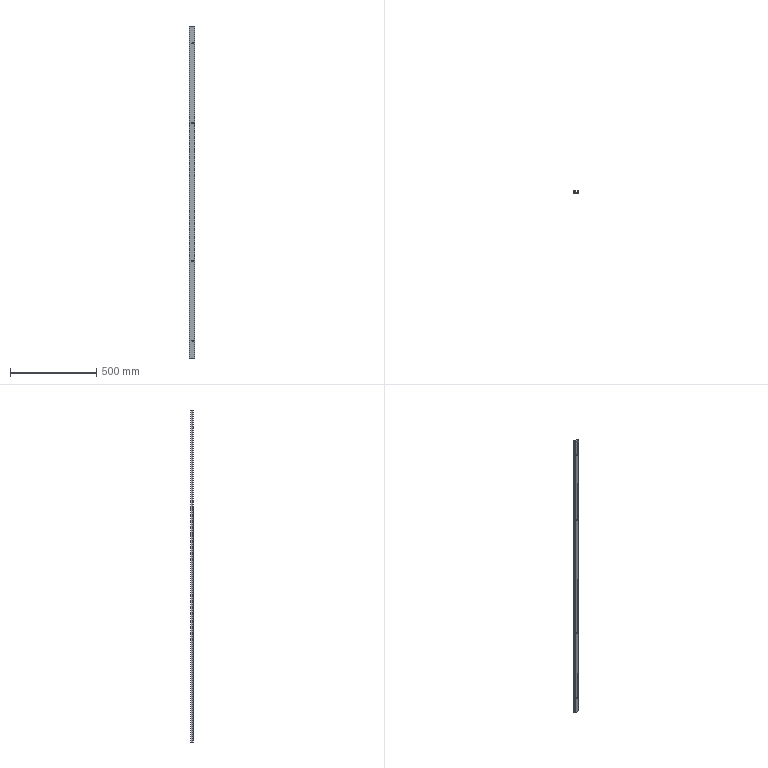Part | SolidWorks | features ICE 2, BaseBody 1, HoleWzd 1, MoveFace 1 | 1 solid | 35 faces | box 33.5 x 13.5 x 1920 mm | volume 359220 mm3 | plane 17 | cylinder 10 | cone 8 | commonest cylinder face diameters 13.44 x4 2 x3 4 x2 1.5 x1
STEP:
#1=CARTESIAN_POINT('',(20.,0.,1723.72));
#2=VERTEX_POINT('',#1);
#3=CARTESIAN_POINT('',(20.,0.,1716.28));
#4=VERTEX_POINT('',#3);
#5=CARTESIAN_POINT('',(20.,0.,1720.));
#6=DIRECTION('',(0.,-1.,0.));
#7=DIRECTION('',(0.,0.,-1.));
#8=AXIS2_PLACEMENT_3D('',#5,#6,#7);
#9=CIRCLE('',#8,3.72);
#10=EDGE_CURVE('',#2,#4,#9,.T.);
#11=ORIENTED_EDGE('',*,*,#10,.T.);
#12=CARTESIAN_POINT('',(20.,3.,1713.28));
#13=VERTEX_POINT('',#12);
#14=CARTESIAN_POINT('',(20.,3.,1713.28));
#15=DIRECTION('',(0.,0.7071,-0.7071));
#16=VECTOR('',#15,1000.);
#17=LINE('',#14,#16);
#18=EDGE_CURVE('',#4,#13,#17,.T.);
#19=ORIENTED_EDGE('',*,*,#18,.T.);
#20=CARTESIAN_POINT('',(20.,3.,1726.72));
#21=VERTEX_POINT('',#20);
#22=CARTESIAN_POINT('',(20.,3.,1720.));
#23=DIRECTION('',(0.,1.,0.));
#24=DIRECTION('',(0.,0.,1.));
#25=AXIS2_PLACEMENT_3D('',#22,#23,#24);
#26=CIRCLE('',#25,6.72);
#27=EDGE_CURVE('',#13,#21,#26,.T.);
#28=ORIENTED_EDGE('',*,*,#27,.T.);
#29=CARTESIAN_POINT('',(20.,3.,1726.72));
#30=DIRECTION('',(0.,0.7071,0.7071));
#31=VECTOR('',#30,1000.);
#32=LINE('',#29,#31);
#33=EDGE_CURVE('',#2,#21,#32,.T.);
#34=ORIENTED_EDGE('',*,*,#33,.F.);
#35=EDGE_LOOP('',(#11,#19,#28,#34));
#36=FACE_OUTER_BOUND('',#35,.T.);
#37=CARTESIAN_POINT('',(20.,3.,1720.));
#38=DIRECTION('',(0.,1.,0.));
#39=DIRECTION('',(0.,0.,1.));
#40=AXIS2_PLACEMENT_3D('',#37,#38,#39);
#41=CONICAL_SURFACE('',#40,6.72,0.7854);
#42=ADVANCED_FACE('',(#36),#41,.F.);
#43=CARTESIAN_POINT('',(20.,0.,3.72));
#44=VERTEX_POINT('',#43);
#45=CARTESIAN_POINT('',(20.,0.,-3.72));
#46=VERTEX_POINT('',#45);
#47=CARTESIAN_POINT('',(20.,0.,0.));
#48=DIRECTION('',(0.,-1.,0.));
#49=DIRECTION('',(0.,0.,-1.));
#50=AXIS2_PLACEMENT_3D('',#47,#48,#49);
#51=CIRCLE('',#50,3.72);
#52=EDGE_CURVE('',#44,#46,#51,.T.);
#53=ORIENTED_EDGE('',*,*,#52,.T.);
#54=CARTESIAN_POINT('',(20.,3.,-6.72));
#55=VERTEX_POINT('',#54);
#56=CARTESIAN_POINT('',(20.,3.,-6.72));
#57=DIRECTION('',(0.,0.7071,-0.7071));
#58=VECTOR('',#57,1000.);
#59=LINE('',#56,#58);
#60=EDGE_CURVE('',#46,#55,#59,.T.);
#61=ORIENTED_EDGE('',*,*,#60,.T.);
#62=CARTESIAN_POINT('',(20.,3.,6.72));
#63=VERTEX_POINT('',#62);
#64=CARTESIAN_POINT('',(20.,3.,0.));
#65=DIRECTION('',(0.,1.,0.));
#66=DIRECTION('',(0.,0.,1.));
#67=AXIS2_PLACEMENT_3D('',#64,#65,#66);
#68=CIRCLE('',#67,6.72);
#69=EDGE_CURVE('',#55,#63,#68,.T.);
#70=ORIENTED_EDGE('',*,*,#69,.T.);
#71=CARTESIAN_POINT('',(20.,3.,6.72));
#72=DIRECTION('',(0.,0.7071,0.7071));
#73=VECTOR('',#72,1000.);
#74=LINE('',#71,#73);
#75=EDGE_CURVE('',#44,#63,#74,.T.);
#76=ORIENTED_EDGE('',*,*,#75,.F.);
#77=EDGE_LOOP('',(#53,#61,#70,#76));
#78=FACE_OUTER_BOUND('',#77,.T.);
#79=CARTESIAN_POINT('',(20.,3.,0.));
#80=DIRECTION('',(0.,1.,0.));
#81=DIRECTION('',(0.,0.,1.));
#82=AXIS2_PLACEMENT_3D('',#79,#80,#81);
#83=CONICAL_SURFACE('',#82,6.72,0.7854);
#84=ADVANCED_FACE('',(#78),#83,.F.);
#85=CARTESIAN_POINT('',(20.,0.,463.72));
#86=VERTEX_POINT('',#85);
#87=CARTESIAN_POINT('',(20.,0.,456.28));
#88=VERTEX_POINT('',#87);
#89=CARTESIAN_POINT('',(20.,0.,460.));
#90=DIRECTION('',(0.,-1.,0.));
#91=DIRECTION('',(0.,0.,-1.));
#92=AXIS2_PLACEMENT_3D('',#89,#90,#91);
#93=CIRCLE('',#92,3.72);
#94=EDGE_CURVE('',#86,#88,#93,.T.);
#95=ORIENTED_EDGE('',*,*,#94,.T.);
#96=CARTESIAN_POINT('',(20.,3.,453.28));
#97=VERTEX_POINT('',#96);
#98=CARTESIAN_POINT('',(20.,3.,453.28));
#99=DIRECTION('',(0.,0.7071,-0.7071));
#100=VECTOR('',#99,1000.);
#101=LINE('',#98,#100);
#102=EDGE_CURVE('',#88,#97,#101,.T.);
#103=ORIENTED_EDGE('',*,*,#102,.T.);
#104=CARTESIAN_POINT('',(20.,3.,466.72));
#105=VERTEX_POINT('',#104);
#106=CARTESIAN_POINT('',(20.,3.,460.));
#107=DIRECTION('',(0.,1.,0.));
#108=DIRECTION('',(0.,0.,1.));
#109=AXIS2_PLACEMENT_3D('',#106,#107,#108);
#110=CIRCLE('',#109,6.72);
#111=EDGE_CURVE('',#97,#105,#110,.T.);
#112=ORIENTED_EDGE('',*,*,#111,.T.);
#113=CARTESIAN_POINT('',(20.,3.,466.72));
#114=DIRECTION('',(0.,0.7071,0.7071));
#115=VECTOR('',#114,1000.);
#116=LINE('',#113,#115);
#117=EDGE_CURVE('',#86,#105,#116,.T.);
#118=ORIENTED_EDGE('',*,*,#117,.F.);
#119=EDGE_LOOP('',(#95,#103,#112,#118));
#120=FACE_OUTER_BOUND('',#119,.T.);
#121=CARTESIAN_POINT('',(20.,3.,460.));
#122=DIRECTION('',(0.,1.,0.));
#123=DIRECTION('',(0.,0.,1.));
#124=AXIS2_PLACEMENT_3D('',#121,#122,#123);
#125=CONICAL_SURFACE('',#124,6.72,0.7854);
#126=ADVANCED_FACE('',(#120),#125,.F.);
#127=CARTESIAN_POINT('',(20.,0.,1263.72));
#128=VERTEX_POINT('',#127);
#129=CARTESIAN_POINT('',(20.,0.,1256.28));
#130=VERTEX_POINT('',#129);
#131=CARTESIAN_POINT('',(20.,0.,1260.));
#132=DIRECTION('',(0.,-1.,0.));
#133=DIRECTION('',(0.,0.,-1.));
#134=AXIS2_PLACEMENT_3D('',#131,#132,#133);
#135=CIRCLE('',#134,3.72);
#136=EDGE_CURVE('',#128,#130,#135,.T.);
#137=ORIENTED_EDGE('',*,*,#136,.T.);
#138=CARTESIAN_POINT('',(20.,3.,1253.28));
#139=VERTEX_POINT('',#138);
#140=CARTESIAN_POINT('',(20.,3.,1253.28));
#141=DIRECTION('',(0.,0.7071,-0.7071));
#142=VECTOR('',#141,1000.);
#143=LINE('',#140,#142);
#144=EDGE_CURVE('',#130,#139,#143,.T.);
#145=ORIENTED_EDGE('',*,*,#144,.T.);
#146=CARTESIAN_POINT('',(20.,3.,1266.72));
#147=VERTEX_POINT('',#146);
#148=CARTESIAN_POINT('',(20.,3.,1260.));
#149=DIRECTION('',(0.,1.,0.));
#150=DIRECTION('',(0.,0.,1.));
#151=AXIS2_PLACEMENT_3D('',#148,#149,#150);
#152=CIRCLE('',#151,6.72);
#153=EDGE_CURVE('',#139,#147,#152,.T.);
#154=ORIENTED_EDGE('',*,*,#153,.T.);
#155=CARTESIAN_POINT('',(20.,3.,1266.72));
#156=DIRECTION('',(0.,0.7071,0.7071));
#157=VECTOR('',#156,1000.);
#158=LINE('',#155,#157);
#159=EDGE_CURVE('',#128,#147,#158,.T.);
#160=ORIENTED_EDGE('',*,*,#159,.F.);
#161=EDGE_LOOP('',(#137,#145,#154,#160));
#162=FACE_OUTER_BOUND('',#161,.T.);
#163=CARTESIAN_POINT('',(20.,3.,1260.));
#164=DIRECTION('',(0.,1.,0.));
#165=DIRECTION('',(0.,0.,1.));
#166=AXIS2_PLACEMENT_3D('',#163,#164,#165);
#167=CONICAL_SURFACE('',#166,6.72,0.7854);
#168=ADVANCED_FACE('',(#162),#167,.F.);
#169=CARTESIAN_POINT('',(24.5,10.5,1255.009));
#170=VERTEX_POINT('',#169);
#171=CARTESIAN_POINT('',(24.5,10.5,464.991));
#172=VERTEX_POINT('',#171);
#173=CARTESIAN_POINT('',(24.5,10.5,-100.));
#174=DIRECTION('',(0.,0.,-1.));
#175=VECTOR('',#174,1000.);
#176=LINE('',#173,#175);
#177=EDGE_CURVE('',#170,#172,#176,.T.);
#178=ORIENTED_EDGE('',*,*,#177,.F.);
#179=CARTESIAN_POINT('',(24.5,10.5,1264.991));
#180=VERTEX_POINT('',#179);
#181=CARTESIAN_POINT('',(24.5,10.5,1255.009));
#182=CARTESIAN_POINT('',(24.5,10.64,1255.009));
#183=CARTESIAN_POINT('',(24.514,10.776,1255.022));
#184=CARTESIAN_POINT('',(24.57,11.042,1255.073));
#185=CARTESIAN_POINT('',(24.611,11.171,1255.111));
#186=CARTESIAN_POINT('',(24.713,11.408,1255.209));
#187=CARTESIAN_POINT('',(24.775,11.519,1255.27));
#188=CARTESIAN_POINT('',(24.908,11.717,1255.409));
#189=CARTESIAN_POINT('',(24.981,11.806,1255.488));
#190=CARTESIAN_POINT('',(25.207,12.042,1255.746));
#191=CARTESIAN_POINT('',(25.363,12.155,1255.942));
#192=CARTESIAN_POINT('',(25.665,12.326,1256.376));
#193=CARTESIAN_POINT('',(25.806,12.38,1256.605));
#194=CARTESIAN_POINT('',(26.061,12.456,1257.084));
#195=CARTESIAN_POINT('',(26.176,12.476,1257.337));
#196=CARTESIAN_POINT('',(26.372,12.498,1257.849));
#197=CARTESIAN_POINT('',(26.454,12.501,1258.109));
#198=CARTESIAN_POINT('',(26.586,12.499,1258.638));
#199=CARTESIAN_POINT('',(26.636,12.496,1258.907));
#200=CARTESIAN_POINT('',(26.703,12.49,1259.453));
#201=CARTESIAN_POINT('',(26.72,12.488,1259.729));
#202=CARTESIAN_POINT('',(26.72,12.488,1260.275));
#203=CARTESIAN_POINT('',(26.703,12.49,1260.547));
#204=CARTESIAN_POINT('',(26.637,12.496,1261.089));
#205=CARTESIAN_POINT('',(26.587,12.499,1261.36));
#206=CARTESIAN_POINT('',(26.387,12.501,1262.161));
#207=CARTESIAN_POINT('',(26.191,12.494,1262.671));
#208=CARTESIAN_POINT('',(25.805,12.38,1263.396));
#209=CARTESIAN_POINT('',(25.663,12.325,1263.627));
#210=CARTESIAN_POINT('',(25.364,12.155,1264.057));
#211=CARTESIAN_POINT('',(25.205,12.039,1264.256));
#212=CARTESIAN_POINT('',(24.981,11.805,1264.512));
#213=CARTESIAN_POINT('',(24.907,11.716,1264.592));
#214=CARTESIAN_POINT('',(24.774,11.518,1264.73));
#215=CARTESIAN_POINT('',(24.714,11.409,1264.79));
#216=CARTESIAN_POINT('',(24.611,11.17,1264.889));
#217=CARTESIAN_POINT('',(24.571,11.044,1264.926));
#218=CARTESIAN_POINT('',(24.515,10.78,1264.977));
#219=CARTESIAN_POINT('',(24.5,10.64,1264.991));
#220=CARTESIAN_POINT('',(24.5,10.5,1264.991));
#221=B_SPLINE_CURVE_WITH_KNOTS('',3,(#181,#182,#183,#184,#185,#186,#187,#188,#189,#190,#191,#192,#193,#194,#195,#196,#197,#198,#199,#200,#201,#202,#203,#204,#205,#206,#207,#208,#209,#210,#211,#212,#213,#214,#215,#216,#217,#218,#219,#220),.UNSPECIFIED.,.F.,.F.,(4,2,2,2,2,2,2,2,2,2,2,2,2,2,2,2,2,2,2,4),(0.,0.0004127,0.0008255,0.001238,0.001651,0.002476,0.003302,0.004127,0.004953,0.005778,0.006604,0.007429,0.008255,0.009906,0.01073,0.01156,0.01197,0.01238,0.01279,0.01321),.UNSPECIFIED.);
#222=EDGE_CURVE('',#170,#180,#221,.T.);
#223=ORIENTED_EDGE('',*,*,#222,.T.);
#224=CARTESIAN_POINT('',(24.5,10.5,1715.009));
#225=VERTEX_POINT('',#224);
#226=CARTESIAN_POINT('',(24.5,10.5,-100.));
#227=DIRECTION('',(0.,0.,-1.));
#228=VECTOR('',#227,1000.);
#229=LINE('',#226,#228);
#230=EDGE_CURVE('',#225,#180,#229,.T.);
#231=ORIENTED_EDGE('',*,*,#230,.F.);
#232=CARTESIAN_POINT('',(24.5,10.5,1724.991));
#233=VERTEX_POINT('',#232);
#234=CARTESIAN_POINT('',(24.5,10.5,1715.009));
#235=CARTESIAN_POINT('',(24.5,10.64,1715.009));
#236=CARTESIAN_POINT('',(24.514,10.776,1715.022));
#237=CARTESIAN_POINT('',(24.57,11.042,1715.073));
#238=CARTESIAN_POINT('',(24.611,11.171,1715.111));
#239=CARTESIAN_POINT('',(24.713,11.408,1715.209));
#240=CARTESIAN_POINT('',(24.775,11.519,1715.27));
#241=CARTESIAN_POINT('',(24.908,11.717,1715.409));
#242=CARTESIAN_POINT('',(24.981,11.806,1715.488));
#243=CARTESIAN_POINT('',(25.207,12.042,1715.746));
#244=CARTESIAN_POINT('',(25.363,12.155,1715.942));
#245=CARTESIAN_POINT('',(25.665,12.326,1716.376));
#246=CARTESIAN_POINT('',(25.806,12.38,1716.605));
#247=CARTESIAN_POINT('',(26.061,12.456,1717.084));
#248=CARTESIAN_POINT('',(26.176,12.476,1717.337));
#249=CARTESIAN_POINT('',(26.372,12.498,1717.849));
#250=CARTESIAN_POINT('',(26.454,12.501,1718.109));
#251=CARTESIAN_POINT('',(26.586,12.499,1718.638));
#252=CARTESIAN_POINT('',(26.636,12.496,1718.907));
#253=CARTESIAN_POINT('',(26.703,12.49,1719.453));
#254=CARTESIAN_POINT('',(26.72,12.488,1719.729));
#255=CARTESIAN_POINT('',(26.72,12.488,1720.275));
#256=CARTESIAN_POINT('',(26.703,12.49,1720.547));
#257=CARTESIAN_POINT('',(26.637,12.496,1721.089));
#258=CARTESIAN_POINT('',(26.587,12.499,1721.36));
#259=CARTESIAN_POINT('',(26.387,12.501,1722.161));
#260=CARTESIAN_POINT('',(26.191,12.494,1722.671));
#261=CARTESIAN_POINT('',(25.805,12.38,1723.396));
#262=CARTESIAN_POINT('',(25.663,12.325,1723.627));
#263=CARTESIAN_POINT('',(25.364,12.155,1724.057));
#264=CARTESIAN_POINT('',(25.205,12.039,1724.256));
#265=CARTESIAN_POINT('',(24.981,11.805,1724.512));
#266=CARTESIAN_POINT('',(24.907,11.716,1724.592));
#267=CARTESIAN_POINT('',(24.774,11.518,1724.73));
#268=CARTESIAN_POINT('',(24.714,11.409,1724.79));
#269=CARTESIAN_POINT('',(24.611,11.17,1724.889));
#270=CARTESIAN_POINT('',(24.571,11.044,1724.926));
#271=CARTESIAN_POINT('',(24.515,10.78,1724.977));
#272=CARTESIAN_POINT('',(24.5,10.64,1724.991));
#273=CARTESIAN_POINT('',(24.5,10.5,1724.991));
#274=B_SPLINE_CURVE_WITH_KNOTS('',3,(#234,#235,#236,#237,#238,#239,#240,#241,#242,#243,#244,#245,#246,#247,#248,#249,#250,#251,#252,#253,#254,#255,#256,#257,#258,#259,#260,#261,#262,#263,#264,#265,#266,#267,#268,#269,#270,#271,#272,#273),.UNSPECIFIED.,.F.,.F.,(4,2,2,2,2,2,2,2,2,2,2,2,2,2,2,2,2,2,2,4),(0.,0.0004127,0.0008255,0.001238,0.001651,0.002476,0.003302,0.004127,0.004953,0.005778,0.006604,0.007429,0.008255,0.009906,0.01073,0.01156,0.01197,0.01238,0.01279,0.01321),.UNSPECIFIED.);
#275=EDGE_CURVE('',#225,#233,#274,.T.);
#276=ORIENTED_EDGE('',*,*,#275,.T.);
#277=CARTESIAN_POINT('',(24.5,10.5,1820.));
#278=VERTEX_POINT('',#277);
#279=CARTESIAN_POINT('',(24.5,10.5,-100.));
#280=DIRECTION('',(0.,0.,-1.));
#281=VECTOR('',#280,1000.);
#282=LINE('',#279,#281);
#283=EDGE_CURVE('',#278,#233,#282,.T.);
#284=ORIENTED_EDGE('',*,*,#283,.F.);
#285=CARTESIAN_POINT('',(28.5,10.5,1820.));
#286=VERTEX_POINT('',#285);
#287=CARTESIAN_POINT('',(26.5,10.5,1820.));
#288=DIRECTION('',(0.,0.,1.));
#289=DIRECTION('',(1.,0.,0.));
#290=AXIS2_PLACEMENT_3D('',#287,#288,#289);
#291=CIRCLE('',#290,2.);
#292=EDGE_CURVE('',#286,#278,#291,.T.);
#293=ORIENTED_EDGE('',*,*,#292,.F.);
#294=CARTESIAN_POINT('',(28.5,10.5,-100.));
#295=VERTEX_POINT('',#294);
#296=CARTESIAN_POINT('',(28.5,10.5,-100.));
#297=DIRECTION('',(0.,0.,-1.));
#298=VECTOR('',#297,1000.);
#299=LINE('',#296,#298);
#300=EDGE_CURVE('',#286,#295,#299,.T.);
#301=ORIENTED_EDGE('',*,*,#300,.T.);
#302=CARTESIAN_POINT('',(24.5,10.5,-100.));
#303=VERTEX_POINT('',#302);
#304=CARTESIAN_POINT('',(26.5,10.5,-100.));
#305=DIRECTION('',(0.,0.,1.));
#306=DIRECTION('',(-1.,0.,0.));
#307=AXIS2_PLACEMENT_3D('',#304,#305,#306);
#308=CIRCLE('',#307,2.);
#309=EDGE_CURVE('',#295,#303,#308,.T.);
#310=ORIENTED_EDGE('',*,*,#309,.T.);
#311=CARTESIAN_POINT('',(24.5,10.5,-4.991));
#312=VERTEX_POINT('',#311);
#313=CARTESIAN_POINT('',(24.5,10.5,-100.));
#314=DIRECTION('',(0.,0.,-1.));
#315=VECTOR('',#314,1000.);
#316=LINE('',#313,#315);
#317=EDGE_CURVE('',#312,#303,#316,.T.);
#318=ORIENTED_EDGE('',*,*,#317,.F.);
#319=CARTESIAN_POINT('',(24.5,10.5,4.991));
#320=VERTEX_POINT('',#319);
#321=CARTESIAN_POINT('',(24.5,10.5,-4.991));
#322=CARTESIAN_POINT('',(24.5,10.638,-4.991));
#323=CARTESIAN_POINT('',(24.515,10.777,-4.978));
#324=CARTESIAN_POINT('',(24.57,11.043,-4.927));
#325=CARTESIAN_POINT('',(24.611,11.171,-4.889));
#326=CARTESIAN_POINT('',(24.765,11.529,-4.74));
#327=CARTESIAN_POINT('',(24.907,11.728,-4.597));
#328=CARTESIAN_POINT('',(25.205,12.04,-4.256));
#329=CARTESIAN_POINT('',(25.365,12.156,-4.055));
#330=CARTESIAN_POINT('',(25.663,12.325,-3.627));
#331=CARTESIAN_POINT('',(25.806,12.38,-3.395));
#332=CARTESIAN_POINT('',(26.19,12.494,-2.672));
#333=CARTESIAN_POINT('',(26.387,12.501,-2.161));
#334=CARTESIAN_POINT('',(26.654,12.499,-1.091));
#335=CARTESIAN_POINT('',(26.72,12.488,-0.5481));
#336=CARTESIAN_POINT('',(26.72,12.488,0.2773));
#337=CARTESIAN_POINT('',(26.703,12.49,0.5529));
#338=CARTESIAN_POINT('',(26.636,12.496,1.095));
#339=CARTESIAN_POINT('',(26.586,12.499,1.362));
#340=CARTESIAN_POINT('',(26.388,12.501,2.155));
#341=CARTESIAN_POINT('',(26.188,12.493,2.677));
#342=CARTESIAN_POINT('',(25.805,12.38,3.396));
#343=CARTESIAN_POINT('',(25.662,12.324,3.629));
#344=CARTESIAN_POINT('',(25.438,12.197,3.95));
#345=CARTESIAN_POINT('',(25.362,12.147,4.053));
#346=CARTESIAN_POINT('',(25.208,12.03,4.249));
#347=CARTESIAN_POINT('',(25.13,11.961,4.342));
#348=CARTESIAN_POINT('',(24.98,11.805,4.513));
#349=CARTESIAN_POINT('',(24.908,11.717,4.591));
#350=CARTESIAN_POINT('',(24.774,11.518,4.73));
#351=CARTESIAN_POINT('',(24.714,11.408,4.79));
#352=CARTESIAN_POINT('',(24.612,11.172,4.888));
#353=CARTESIAN_POINT('',(24.57,11.043,4.927));
#354=CARTESIAN_POINT('',(24.515,10.778,4.978));
#355=CARTESIAN_POINT('',(24.5,10.64,4.991));
#356=CARTESIAN_POINT('',(24.5,10.5,4.991));
#357=B_SPLINE_CURVE_WITH_KNOTS('',3,(#321,#322,#323,#324,#325,#326,#327,#328,#329,#330,#331,#332,#333,#334,#335,#336,#337,#338,#339,#340,#341,#342,#343,#344,#345,#346,#347,#348,#349,#350,#351,#352,#353,#354,#355,#356),.UNSPECIFIED.,.F.,.F.,(4,2,2,2,2,2,2,2,2,2,2,2,2,2,2,2,2,4),(0.01321,0.01362,0.01403,0.01486,0.01569,0.01651,0.01816,0.01981,0.02064,0.02146,0.02311,0.02394,0.02435,0.02477,0.02518,0.02559,0.026,0.02642),.UNSPECIFIED.);
#358=EDGE_CURVE('',#312,#320,#357,.T.);
#359=ORIENTED_EDGE('',*,*,#358,.T.);
#360=CARTESIAN_POINT('',(24.5,10.5,455.009));
#361=VERTEX_POINT('',#360);
#362=CARTESIAN_POINT('',(24.5,10.5,-100.));
#363=DIRECTION('',(0.,0.,-1.));
#364=VECTOR('',#363,1000.);
#365=LINE('',#362,#364);
#366=EDGE_CURVE('',#361,#320,#365,.T.);
#367=ORIENTED_EDGE('',*,*,#366,.F.);
#368=CARTESIAN_POINT('',(24.5,10.5,455.009));
#369=CARTESIAN_POINT('',(24.5,10.638,455.009));
#370=CARTESIAN_POINT('',(24.515,10.777,455.022));
#371=CARTESIAN_POINT('',(24.57,11.043,455.073));
#372=CARTESIAN_POINT('',(24.611,11.171,455.111));
#373=CARTESIAN_POINT('',(24.765,11.529,455.26));
#374=CARTESIAN_POINT('',(24.907,11.728,455.403));
#375=CARTESIAN_POINT('',(25.205,12.04,455.744));
#376=CARTESIAN_POINT('',(25.365,12.156,455.945));
#377=CARTESIAN_POINT('',(25.663,12.325,456.373));
#378=CARTESIAN_POINT('',(25.806,12.38,456.605));
#379=CARTESIAN_POINT('',(26.19,12.494,457.328));
#380=CARTESIAN_POINT('',(26.387,12.501,457.839));
#381=CARTESIAN_POINT('',(26.654,12.499,458.909));
#382=CARTESIAN_POINT('',(26.72,12.488,459.452));
#383=CARTESIAN_POINT('',(26.72,12.488,460.277));
#384=CARTESIAN_POINT('',(26.703,12.49,460.553));
#385=CARTESIAN_POINT('',(26.636,12.496,461.095));
#386=CARTESIAN_POINT('',(26.586,12.499,461.362));
#387=CARTESIAN_POINT('',(26.388,12.501,462.155));
#388=CARTESIAN_POINT('',(26.188,12.493,462.677));
#389=CARTESIAN_POINT('',(25.805,12.38,463.396));
#390=CARTESIAN_POINT('',(25.662,12.324,463.629));
#391=CARTESIAN_POINT('',(25.438,12.197,463.95));
#392=CARTESIAN_POINT('',(25.362,12.147,464.053));
#393=CARTESIAN_POINT('',(25.208,12.03,464.249));
#394=CARTESIAN_POINT('',(25.13,11.961,464.342));
#395=CARTESIAN_POINT('',(24.98,11.805,464.513));
#396=CARTESIAN_POINT('',(24.908,11.717,464.591));
#397=CARTESIAN_POINT('',(24.774,11.518,464.73));
#398=CARTESIAN_POINT('',(24.714,11.408,464.79));
#399=CARTESIAN_POINT('',(24.612,11.172,464.888));
#400=CARTESIAN_POINT('',(24.57,11.043,464.927));
#401=CARTESIAN_POINT('',(24.515,10.778,464.978));
#402=CARTESIAN_POINT('',(24.5,10.64,464.991));
#403=CARTESIAN_POINT('',(24.5,10.5,464.991));
#404=B_SPLINE_CURVE_WITH_KNOTS('',3,(#368,#369,#370,#371,#372,#373,#374,#375,#376,#377,#378,#379,#380,#381,#382,#383,#384,#385,#386,#387,#388,#389,#390,#391,#392,#393,#394,#395,#396,#397,#398,#399,#400,#401,#402,#403),.UNSPECIFIED.,.F.,.F.,(4,2,2,2,2,2,2,2,2,2,2,2,2,2,2,2,2,4),(0.01321,0.01362,0.01403,0.01486,0.01569,0.01651,0.01816,0.01981,0.02064,0.02146,0.02311,0.02394,0.02435,0.02477,0.02518,0.02559,0.026,0.02642),.UNSPECIFIED.);
#405=EDGE_CURVE('',#361,#172,#404,.T.);
#406=ORIENTED_EDGE('',*,*,#405,.T.);
#407=EDGE_LOOP('',(#178,#223,#231,#276,#284,#293,#301,#310,#318,#359,#367,#406));
#408=FACE_OUTER_BOUND('',#407,.T.);
#409=CARTESIAN_POINT('',(26.5,10.5,-100.));
#410=DIRECTION('',(0.,0.,-1.));
#411=DIRECTION('',(-1.,0.,0.));
#412=AXIS2_PLACEMENT_3D('',#409,#410,#411);
#413=CYLINDRICAL_SURFACE('',#412,2.);
#414=ADVANCED_FACE('',(#408),#413,.T.);
#415=CARTESIAN_POINT('',(24.5,3.,1255.009));
#416=VERTEX_POINT('',#415);
#417=CARTESIAN_POINT('',(24.5,3.,464.991));
#418=VERTEX_POINT('',#417);
#419=CARTESIAN_POINT('',(24.5,3.,-100.));
#420=DIRECTION('',(0.,0.,-1.));
#421=VECTOR('',#420,1000.);
#422=LINE('',#419,#421);
#423=EDGE_CURVE('',#416,#418,#422,.T.);
#424=ORIENTED_EDGE('',*,*,#423,.F.);
#425=CARTESIAN_POINT('',(24.5,48.,1255.009));
#426=DIRECTION('',(0.,1.,0.));
#427=VECTOR('',#426,1000.);
#428=LINE('',#425,#427);
#429=EDGE_CURVE('',#416,#170,#428,.T.);
#430=ORIENTED_EDGE('',*,*,#429,.T.);
#431=ORIENTED_EDGE('',*,*,#177,.T.);
#432=CARTESIAN_POINT('',(24.5,13.5,464.991));
#433=DIRECTION('',(0.,-1.,0.));
#434=VECTOR('',#433,1000.);
#435=LINE('',#432,#434);
#436=EDGE_CURVE('',#172,#418,#435,.T.);
#437=ORIENTED_EDGE('',*,*,#436,.T.);
#438=EDGE_LOOP('',(#424,#430,#431,#437));
#439=FACE_OUTER_BOUND('',#438,.T.);
#440=CARTESIAN_POINT('',(24.5,10.5,-100.));
#441=DIRECTION('',(-1.,0.,0.));
#442=DIRECTION('',(0.,0.,1.));
#443=AXIS2_PLACEMENT_3D('',#440,#441,#442);
#444=PLANE('',#443);
#445=ADVANCED_FACE('',(#439),#444,.T.);
#446=ORIENTED_EDGE('',*,*,#230,.T.);
#447=CARTESIAN_POINT('',(24.5,3.,1264.991));
#448=VERTEX_POINT('',#447);
#449=CARTESIAN_POINT('',(24.5,48.,1264.991));
#450=DIRECTION('',(0.,-1.,0.));
#451=VECTOR('',#450,1000.);
#452=LINE('',#449,#451);
#453=EDGE_CURVE('',#180,#448,#452,.T.);
#454=ORIENTED_EDGE('',*,*,#453,.T.);
#455=CARTESIAN_POINT('',(24.5,3.,1715.009));
#456=VERTEX_POINT('',#455);
#457=CARTESIAN_POINT('',(24.5,3.,-100.));
#458=DIRECTION('',(0.,0.,-1.));
#459=VECTOR('',#458,1000.);
#460=LINE('',#457,#459);
#461=EDGE_CURVE('',#456,#448,#460,.T.);
#462=ORIENTED_EDGE('',*,*,#461,.F.);
#463=CARTESIAN_POINT('',(24.5,13.5,1715.009));
#464=DIRECTION('',(0.,1.,0.));
#465=VECTOR('',#464,1000.);
#466=LINE('',#463,#465);
#467=EDGE_CURVE('',#456,#225,#466,.T.);
#468=ORIENTED_EDGE('',*,*,#467,.T.);
#469=EDGE_LOOP('',(#446,#454,#462,#468));
#470=FACE_OUTER_BOUND('',#469,.T.);
#471=CARTESIAN_POINT('',(24.5,10.5,-100.));
#472=DIRECTION('',(-1.,0.,0.));
#473=DIRECTION('',(0.,0.,1.));
#474=AXIS2_PLACEMENT_3D('',#471,#472,#473);
#475=PLANE('',#474);
#476=ADVANCED_FACE('',(#470),#475,.T.);
#477=CARTESIAN_POINT('',(24.5,3.,-4.991));
#478=VERTEX_POINT('',#477);
#479=CARTESIAN_POINT('',(24.5,3.,-100.));
#480=VERTEX_POINT('',#479);
#481=CARTESIAN_POINT('',(24.5,3.,-100.));
#482=DIRECTION('',(0.,0.,-1.));
#483=VECTOR('',#482,1000.);
#484=LINE('',#481,#483);
#485=EDGE_CURVE('',#478,#480,#484,.T.);
#486=ORIENTED_EDGE('',*,*,#485,.F.);
#487=CARTESIAN_POINT('',(24.5,13.5,-4.991));
#488=DIRECTION('',(0.,1.,0.));
#489=VECTOR('',#488,1000.);
#490=LINE('',#487,#489);
#491=EDGE_CURVE('',#478,#312,#490,.T.);
#492=ORIENTED_EDGE('',*,*,#491,.T.);
#493=ORIENTED_EDGE('',*,*,#317,.T.);
#494=CARTESIAN_POINT('',(24.5,1.,-100.));
#495=DIRECTION('',(0.,-1.,0.));
#496=VECTOR('',#495,1000.);
#497=LINE('',#494,#496);
#498=EDGE_CURVE('',#303,#480,#497,.T.);
#499=ORIENTED_EDGE('',*,*,#498,.T.);
#500=EDGE_LOOP('',(#486,#492,#493,#499));
#501=FACE_OUTER_BOUND('',#500,.T.);
#502=CARTESIAN_POINT('',(24.5,10.5,-100.));
#503=DIRECTION('',(-1.,0.,0.));
#504=DIRECTION('',(0.,0.,1.));
#505=AXIS2_PLACEMENT_3D('',#502,#503,#504);
#506=PLANE('',#505);
#507=ADVANCED_FACE('',(#501),#506,.T.);
#508=ORIENTED_EDGE('',*,*,#366,.T.);
#509=CARTESIAN_POINT('',(24.5,3.,4.991));
#510=VERTEX_POINT('',#509);
#511=CARTESIAN_POINT('',(24.5,13.5,4.991));
#512=DIRECTION('',(0.,-1.,0.));
#513=VECTOR('',#512,1000.);
#514=LINE('',#511,#513);
#515=EDGE_CURVE('',#320,#510,#514,.T.);
#516=ORIENTED_EDGE('',*,*,#515,.T.);
#517=CARTESIAN_POINT('',(24.5,3.,455.009));
#518=VERTEX_POINT('',#517);
#519=CARTESIAN_POINT('',(24.5,3.,-100.));
#520=DIRECTION('',(0.,0.,-1.));
#521=VECTOR('',#520,1000.);
#522=LINE('',#519,#521);
#523=EDGE_CURVE('',#518,#510,#522,.T.);
#524=ORIENTED_EDGE('',*,*,#523,.F.);
#525=CARTESIAN_POINT('',(24.5,13.5,455.009));
#526=DIRECTION('',(0.,1.,0.));
#527=VECTOR('',#526,1000.);
#528=LINE('',#525,#527);
#529=EDGE_CURVE('',#518,#361,#528,.T.);
#530=ORIENTED_EDGE('',*,*,#529,.T.);
#531=EDGE_LOOP('',(#508,#516,#524,#530));
#532=FACE_OUTER_BOUND('',#531,.T.);
#533=CARTESIAN_POINT('',(24.5,10.5,-100.));
#534=DIRECTION('',(-1.,0.,0.));
#535=DIRECTION('',(0.,0.,1.));
#536=AXIS2_PLACEMENT_3D('',#533,#534,#535);
#537=PLANE('',#536);
#538=ADVANCED_FACE('',(#532),#537,.T.);
#539=ORIENTED_EDGE('',*,*,#283,.T.);
#540=CARTESIAN_POINT('',(24.5,3.,1724.991));
#541=VERTEX_POINT('',#540);
#542=CARTESIAN_POINT('',(24.5,13.5,1724.991));
#543=DIRECTION('',(0.,-1.,0.));
#544=VECTOR('',#543,1000.);
#545=LINE('',#542,#544);
#546=EDGE_CURVE('',#233,#541,#545,.T.);
#547=ORIENTED_EDGE('',*,*,#546,.T.);
#548=CARTESIAN_POINT('',(24.5,3.,1820.));
#549=VERTEX_POINT('',#548);
#550=CARTESIAN_POINT('',(24.5,3.,-100.));
#551=DIRECTION('',(0.,0.,-1.));
#552=VECTOR('',#551,1000.);
#553=LINE('',#550,#552);
#554=EDGE_CURVE('',#549,#541,#553,.T.);
#555=ORIENTED_EDGE('',*,*,#554,.F.);
#556=CARTESIAN_POINT('',(24.5,1.,1820.));
#557=DIRECTION('',(0.,-1.,0.));
#558=VECTOR('',#557,1000.);
#559=LINE('',#556,#558);
#560=EDGE_CURVE('',#278,#549,#559,.T.);
#561=ORIENTED_EDGE('',*,*,#560,.F.);
#562=EDGE_LOOP('',(#539,#547,#555,#561));
#563=FACE_OUTER_BOUND('',#562,.T.);
#564=CARTESIAN_POINT('',(24.5,10.5,-100.));
#565=DIRECTION('',(-1.,0.,0.));
#566=DIRECTION('',(0.,0.,1.));
#567=AXIS2_PLACEMENT_3D('',#564,#565,#566);
#568=PLANE('',#567);
#569=ADVANCED_FACE('',(#563),#568,.T.);
#570=ORIENTED_EDGE('',*,*,#10,.F.);
#571=CARTESIAN_POINT('',(20.,0.,1720.));
#572=DIRECTION('',(0.,-1.,0.));
#573=DIRECTION('',(0.,0.,-1.));
#574=AXIS2_PLACEMENT_3D('',#571,#572,#573);
#575=CIRCLE('',#574,3.72);
#576=EDGE_CURVE('',#4,#2,#575,.T.);
#577=ORIENTED_EDGE('',*,*,#576,.F.);
#578=EDGE_LOOP('',(#570,#577));
#579=FACE_BOUND('',#578,.T.);
#580=ORIENTED_EDGE('',*,*,#52,.F.);
#581=CARTESIAN_POINT('',(20.,0.,0.));
#582=DIRECTION('',(0.,-1.,0.));
#583=DIRECTION('',(0.,0.,-1.));
#584=AXIS2_PLACEMENT_3D('',#581,#582,#583);
#585=CIRCLE('',#584,3.72);
#586=EDGE_CURVE('',#46,#44,#585,.T.);
#587=ORIENTED_EDGE('',*,*,#586,.F.);
#588=EDGE_LOOP('',(#580,#587));
#589=FACE_BOUND('',#588,.T.);
#590=ORIENTED_EDGE('',*,*,#94,.F.);
#591=CARTESIAN_POINT('',(20.,0.,460.));
#592=DIRECTION('',(0.,-1.,0.));
#593=DIRECTION('',(0.,0.,-1.));
#594=AXIS2_PLACEMENT_3D('',#591,#592,#593);
#595=CIRCLE('',#594,3.72);
#596=EDGE_CURVE('',#88,#86,#595,.T.);
#597=ORIENTED_EDGE('',*,*,#596,.F.);
#598=EDGE_LOOP('',(#590,#597));
#599=FACE_BOUND('',#598,.T.);
#600=CARTESIAN_POINT('',(1.,0.,-100.));
#601=VERTEX_POINT('',#600);
#602=CARTESIAN_POINT('',(32.5,0.,-100.));
#603=VERTEX_POINT('',#602);
#604=CARTESIAN_POINT('',(1.,0.,-100.));
#605=DIRECTION('',(1.,0.,0.));
#606=VECTOR('',#605,1000.);
#607=LINE('',#604,#606);
#608=EDGE_CURVE('',#601,#603,#607,.T.);
#609=ORIENTED_EDGE('',*,*,#608,.T.);
#610=CARTESIAN_POINT('',(32.5,0.,1820.));
#611=VERTEX_POINT('',#610);
#612=CARTESIAN_POINT('',(32.5,0.,-100.));
#613=DIRECTION('',(0.,0.,1.));
#614=VECTOR('',#613,1000.);
#615=LINE('',#612,#614);
#616=EDGE_CURVE('',#603,#611,#615,.T.);
#617=ORIENTED_EDGE('',*,*,#616,.T.);
#618=CARTESIAN_POINT('',(1.,0.,1820.));
#619=VERTEX_POINT('',#618);
#620=CARTESIAN_POINT('',(1.,0.,1820.));
#621=DIRECTION('',(-1.,0.,0.));
#622=VECTOR('',#621,1000.);
#623=LINE('',#620,#622);
#624=EDGE_CURVE('',#611,#619,#623,.T.);
#625=ORIENTED_EDGE('',*,*,#624,.T.);
#626=CARTESIAN_POINT('',(1.,0.,-100.));
#627=DIRECTION('',(0.,0.,-1.));
#628=VECTOR('',#627,1000.);
#629=LINE('',#626,#628);
#630=EDGE_CURVE('',#619,#601,#629,.T.);
#631=ORIENTED_EDGE('',*,*,#630,.T.);
#632=EDGE_LOOP('',(#609,#617,#625,#631));
#633=FACE_OUTER_BOUND('',#632,.T.);
#634=ORIENTED_EDGE('',*,*,#136,.F.);
#635=CARTESIAN_POINT('',(20.,0.,1260.));
#636=DIRECTION('',(0.,-1.,0.));
#637=DIRECTION('',(0.,0.,-1.));
#638=AXIS2_PLACEMENT_3D('',#635,#636,#637);
#639=CIRCLE('',#638,3.72);
#640=EDGE_CURVE('',#130,#128,#639,.T.);
#641=ORIENTED_EDGE('',*,*,#640,.F.);
#642=EDGE_LOOP('',(#634,#641));
#643=FACE_BOUND('',#642,.T.);
#644=CARTESIAN_POINT('',(1.,0.,-100.));
#645=DIRECTION('',(0.,-1.,0.));
#646=DIRECTION('',(0.,0.,-1.));
#647=AXIS2_PLACEMENT_3D('',#644,#645,#646);
#648=PLANE('',#647);
#649=ADVANCED_FACE('',(#579,#589,#599,#633,#643),#648,.T.);
#650=CARTESIAN_POINT('',(33.5,1.,-100.));
#651=VERTEX_POINT('',#650);
#652=CARTESIAN_POINT('',(32.5,1.,-100.));
#653=DIRECTION('',(0.,0.,1.));
#654=DIRECTION('',(-1.,0.,0.));
#655=AXIS2_PLACEMENT_3D('',#652,#653,#654);
#656=CIRCLE('',#655,1.);
#657=EDGE_CURVE('',#603,#651,#656,.T.);
#658=ORIENTED_EDGE('',*,*,#657,.T.);
#659=CARTESIAN_POINT('',(33.5,1.,1820.));
#660=VERTEX_POINT('',#659);
#661=CARTESIAN_POINT('',(33.5,1.,-100.));
#662=DIRECTION('',(0.,0.,1.));
#663=VECTOR('',#662,1000.);
#664=LINE('',#661,#663);
#665=EDGE_CURVE('',#651,#660,#664,.T.);
#666=ORIENTED_EDGE('',*,*,#665,.T.);
#667=CARTESIAN_POINT('',(32.5,1.,1820.));
#668=DIRECTION('',(0.,0.,-1.));
#669=DIRECTION('',(1.,0.,0.));
#670=AXIS2_PLACEMENT_3D('',#667,#668,#669);
#671=CIRCLE('',#670,1.);
#672=EDGE_CURVE('',#660,#611,#671,.T.);
#673=ORIENTED_EDGE('',*,*,#672,.T.);
#674=ORIENTED_EDGE('',*,*,#616,.F.);
#675=EDGE_LOOP('',(#658,#666,#673,#674));
#676=FACE_OUTER_BOUND('',#675,.T.);
#677=CARTESIAN_POINT('',(32.5,1.,-100.));
#678=DIRECTION('',(0.,0.,-1.));
#679=DIRECTION('',(-1.,0.,0.));
#680=AXIS2_PLACEMENT_3D('',#677,#678,#679);
#681=CYLINDRICAL_SURFACE('',#680,1.);
#682=ADVANCED_FACE('',(#676),#681,.T.);
#683=CARTESIAN_POINT('',(1.5,12.75,-100.));
#684=VERTEX_POINT('',#683);
#685=CARTESIAN_POINT('',(0.,12.75,-100.));
#686=VERTEX_POINT('',#685);
#687=CARTESIAN_POINT('',(0.75,12.75,-100.));
#688=DIRECTION('',(0.,0.,1.));
#689=DIRECTION('',(-1.,0.,0.));
#690=AXIS2_PLACEMENT_3D('',#687,#688,#689);
#691=CIRCLE('',#690,0.75);
#692=EDGE_CURVE('',#684,#686,#691,.T.);
#693=ORIENTED_EDGE('',*,*,#692,.F.);
#694=CARTESIAN_POINT('',(1.5,3.,-100.));
#695=VERTEX_POINT('',#694);
#696=CARTESIAN_POINT('',(1.5,1.,-100.));
#697=DIRECTION('',(0.,1.,0.));
#698=VECTOR('',#697,1000.);
#699=LINE('',#696,#698);
#700=EDGE_CURVE('',#695,#684,#699,.T.);
#701=ORIENTED_EDGE('',*,*,#700,.F.);
#702=CARTESIAN_POINT('',(8.5,3.,-100.));
#703=VERTEX_POINT('',#702);
#704=CARTESIAN_POINT('',(1.,3.,-100.));
#705=DIRECTION('',(-1.,0.,0.));
#706=VECTOR('',#705,1000.);
#707=LINE('',#704,#706);
#708=EDGE_CURVE('',#703,#695,#707,.T.);
#709=ORIENTED_EDGE('',*,*,#708,.F.);
#710=CARTESIAN_POINT('',(8.5,10.5,-100.));
#711=VERTEX_POINT('',#710);
#712=CARTESIAN_POINT('',(8.5,1.,-100.));
#713=DIRECTION('',(0.,-1.,0.));
#714=VECTOR('',#713,1000.);
#715=LINE('',#712,#714);
#716=EDGE_CURVE('',#711,#703,#715,.T.);
#717=ORIENTED_EDGE('',*,*,#716,.F.);
#718=CARTESIAN_POINT('',(12.5,10.5,-100.));
#719=VERTEX_POINT('',#718);
#720=CARTESIAN_POINT('',(10.5,10.5,-100.));
#721=DIRECTION('',(0.,0.,1.));
#722=DIRECTION('',(-1.,0.,0.));
#723=AXIS2_PLACEMENT_3D('',#720,#721,#722);
#724=CIRCLE('',#723,2.);
#725=EDGE_CURVE('',#719,#711,#724,.T.);
#726=ORIENTED_EDGE('',*,*,#725,.F.);
#727=CARTESIAN_POINT('',(12.5,3.,-100.));
#728=VERTEX_POINT('',#727);
#729=CARTESIAN_POINT('',(12.5,1.,-100.));
#730=DIRECTION('',(0.,1.,0.));
#731=VECTOR('',#730,1000.);
#732=LINE('',#729,#731);
#733=EDGE_CURVE('',#728,#719,#732,.T.);
#734=ORIENTED_EDGE('',*,*,#733,.F.);
#735=CARTESIAN_POINT('',(1.,3.,-100.));
#736=DIRECTION('',(-1.,0.,0.));
#737=VECTOR('',#736,1000.);
#738=LINE('',#735,#737);
#739=EDGE_CURVE('',#480,#728,#738,.T.);
#740=ORIENTED_EDGE('',*,*,#739,.F.);
#741=ORIENTED_EDGE('',*,*,#498,.F.);
#742=ORIENTED_EDGE('',*,*,#309,.F.);
#743=CARTESIAN_POINT('',(28.5,3.,-100.));
#744=VERTEX_POINT('',#743);
#745=CARTESIAN_POINT('',(28.5,1.,-100.));
#746=DIRECTION('',(0.,1.,0.));
#747=VECTOR('',#746,1000.);
#748=LINE('',#745,#747);
#749=EDGE_CURVE('',#744,#295,#748,.T.);
#750=ORIENTED_EDGE('',*,*,#749,.F.);
#751=CARTESIAN_POINT('',(32.5,3.,-100.));
#752=VERTEX_POINT('',#751);
#753=CARTESIAN_POINT('',(1.,3.,-100.));
#754=DIRECTION('',(-1.,0.,0.));
#755=VECTOR('',#754,1000.);
#756=LINE('',#753,#755);
#757=EDGE_CURVE('',#752,#744,#756,.T.);
#758=ORIENTED_EDGE('',*,*,#757,.F.);
#759=CARTESIAN_POINT('',(33.5,2.,-100.));
#760=VERTEX_POINT('',#759);
#761=CARTESIAN_POINT('',(32.5,2.,-100.));
#762=DIRECTION('',(0.,0.,1.));
#763=DIRECTION('',(-1.,0.,0.));
#764=AXIS2_PLACEMENT_3D('',#761,#762,#763);
#765=CIRCLE('',#764,1.);
#766=EDGE_CURVE('',#760,#752,#765,.T.);
#767=ORIENTED_EDGE('',*,*,#766,.F.);
#768=CARTESIAN_POINT('',(33.5,1.,-100.));
#769=DIRECTION('',(0.,1.,0.));
#770=VECTOR('',#769,1000.);
#771=LINE('',#768,#770);
#772=EDGE_CURVE('',#651,#760,#771,.T.);
#773=ORIENTED_EDGE('',*,*,#772,.F.);
#774=ORIENTED_EDGE('',*,*,#657,.F.);
#775=ORIENTED_EDGE('',*,*,#608,.F.);
#776=CARTESIAN_POINT('',(0.,1.,-100.));
#777=VERTEX_POINT('',#776);
#778=CARTESIAN_POINT('',(1.,1.,-100.));
#779=DIRECTION('',(0.,0.,1.));
#780=DIRECTION('',(-1.,0.,0.));
#781=AXIS2_PLACEMENT_3D('',#778,#779,#780);
#782=CIRCLE('',#781,1.);
#783=EDGE_CURVE('',#777,#601,#782,.T.);
#784=ORIENTED_EDGE('',*,*,#783,.F.);
#785=CARTESIAN_POINT('',(0.,1.,-100.));
#786=DIRECTION('',(0.,-1.,0.));
#787=VECTOR('',#786,1000.);
#788=LINE('',#785,#787);
#789=EDGE_CURVE('',#686,#777,#788,.T.);
#790=ORIENTED_EDGE('',*,*,#789,.F.);
#791=EDGE_LOOP('',(#693,#701,#709,#717,#726,#734,#740,#741,#742,#750,#758,#767,#773,#774,#775,#784,#790));
#792=FACE_OUTER_BOUND('',#791,.T.);
#793=CARTESIAN_POINT('',(1.,1.,-100.));
#794=DIRECTION('',(0.,0.,1.));
#795=DIRECTION('',(1.,0.,0.));
#796=AXIS2_PLACEMENT_3D('',#793,#794,#795);
#797=PLANE('',#796);
#798=ADVANCED_FACE('',(#792),#797,.F.);
#799=ORIENTED_EDGE('',*,*,#783,.T.);
#800=ORIENTED_EDGE('',*,*,#630,.F.);
#801=CARTESIAN_POINT('',(0.,1.,1820.));
#802=VERTEX_POINT('',#801);
#803=CARTESIAN_POINT('',(1.,1.,1820.));
#804=DIRECTION('',(0.,0.,-1.));
#805=DIRECTION('',(1.,0.,0.));
#806=AXIS2_PLACEMENT_3D('',#803,#804,#805);
#807=CIRCLE('',#806,1.);
#808=EDGE_CURVE('',#619,#802,#807,.T.);
#809=ORIENTED_EDGE('',*,*,#808,.T.);
#810=CARTESIAN_POINT('',(0.,1.,-100.));
#811=DIRECTION('',(0.,0.,-1.));
#812=VECTOR('',#811,1000.);
#813=LINE('',#810,#812);
#814=EDGE_CURVE('',#802,#777,#813,.T.);
#815=ORIENTED_EDGE('',*,*,#814,.T.);
#816=EDGE_LOOP('',(#799,#800,#809,#815));
#817=FACE_OUTER_BOUND('',#816,.T.);
#818=CARTESIAN_POINT('',(1.,1.,-100.));
#819=DIRECTION('',(0.,0.,-1.));
#820=DIRECTION('',(-1.,0.,0.));
#821=AXIS2_PLACEMENT_3D('',#818,#819,#820);
#822=CYLINDRICAL_SURFACE('',#821,1.);
#823=ADVANCED_FACE('',(#817),#822,.T.);
#824=CARTESIAN_POINT('',(1.5,3.,1820.));
#825=VERTEX_POINT('',#824);
#826=CARTESIAN_POINT('',(1.5,12.75,1820.));
#827=VERTEX_POINT('',#826);
#828=CARTESIAN_POINT('',(1.5,1.,1820.));
#829=DIRECTION('',(0.,1.,0.));
#830=VECTOR('',#829,1000.);
#831=LINE('',#828,#830);
#832=EDGE_CURVE('',#825,#827,#831,.T.);
#833=ORIENTED_EDGE('',*,*,#832,.T.);
#834=CARTESIAN_POINT('',(0.,12.75,1820.));
#835=VERTEX_POINT('',#834);
#836=CARTESIAN_POINT('',(0.75,12.75,1820.));
#837=DIRECTION('',(0.,0.,1.));
#838=DIRECTION('',(1.,0.,0.));
#839=AXIS2_PLACEMENT_3D('',#836,#837,#838);
#840=CIRCLE('',#839,0.75);
#841=EDGE_CURVE('',#827,#835,#840,.T.);
#842=ORIENTED_EDGE('',*,*,#841,.T.);
#843=CARTESIAN_POINT('',(0.,1.,1820.));
#844=DIRECTION('',(0.,-1.,0.));
#845=VECTOR('',#844,1000.);
#846=LINE('',#843,#845);
#847=EDGE_CURVE('',#835,#802,#846,.T.);
#848=ORIENTED_EDGE('',*,*,#847,.T.);
#849=ORIENTED_EDGE('',*,*,#808,.F.);
#850=ORIENTED_EDGE('',*,*,#624,.F.);
#851=ORIENTED_EDGE('',*,*,#672,.F.);
#852=CARTESIAN_POINT('',(33.5,2.,1820.));
#853=VERTEX_POINT('',#852);
#854=CARTESIAN_POINT('',(33.5,1.,1820.));
#855=DIRECTION('',(0.,1.,0.));
#856=VECTOR('',#855,1000.);
#857=LINE('',#854,#856);
#858=EDGE_CURVE('',#660,#853,#857,.T.);
#859=ORIENTED_EDGE('',*,*,#858,.T.);
#860=CARTESIAN_POINT('',(32.5,3.,1820.));
#861=VERTEX_POINT('',#860);
#862=CARTESIAN_POINT('',(32.5,2.,1820.));
#863=DIRECTION('',(0.,0.,-1.));
#864=DIRECTION('',(1.,0.,0.));
#865=AXIS2_PLACEMENT_3D('',#862,#863,#864);
#866=CIRCLE('',#865,1.);
#867=EDGE_CURVE('',#861,#853,#866,.T.);
#868=ORIENTED_EDGE('',*,*,#867,.F.);
#869=CARTESIAN_POINT('',(28.5,3.,1820.));
#870=VERTEX_POINT('',#869);
#871=CARTESIAN_POINT('',(1.,3.,1820.));
#872=DIRECTION('',(-1.,0.,0.));
#873=VECTOR('',#872,1000.);
#874=LINE('',#871,#873);
#875=EDGE_CURVE('',#861,#870,#874,.T.);
#876=ORIENTED_EDGE('',*,*,#875,.T.);
#877=CARTESIAN_POINT('',(28.5,1.,1820.));
#878=DIRECTION('',(0.,1.,0.));
#879=VECTOR('',#878,1000.);
#880=LINE('',#877,#879);
#881=EDGE_CURVE('',#870,#286,#880,.T.);
#882=ORIENTED_EDGE('',*,*,#881,.T.);
#883=ORIENTED_EDGE('',*,*,#292,.T.);
#884=ORIENTED_EDGE('',*,*,#560,.T.);
#885=CARTESIAN_POINT('',(12.5,3.,1820.));
#886=VERTEX_POINT('',#885);
#887=CARTESIAN_POINT('',(1.,3.,1820.));
#888=DIRECTION('',(-1.,0.,0.));
#889=VECTOR('',#888,1000.);
#890=LINE('',#887,#889);
#891=EDGE_CURVE('',#549,#886,#890,.T.);
#892=ORIENTED_EDGE('',*,*,#891,.T.);
#893=CARTESIAN_POINT('',(12.5,10.5,1820.));
#894=VERTEX_POINT('',#893);
#895=CARTESIAN_POINT('',(12.5,1.,1820.));
#896=DIRECTION('',(0.,1.,0.));
#897=VECTOR('',#896,1000.);
#898=LINE('',#895,#897);
#899=EDGE_CURVE('',#886,#894,#898,.T.);
#900=ORIENTED_EDGE('',*,*,#899,.T.);
#901=CARTESIAN_POINT('',(8.5,10.5,1820.));
#902=VERTEX_POINT('',#901);
#903=CARTESIAN_POINT('',(10.5,10.5,1820.));
#904=DIRECTION('',(0.,0.,1.));
#905=DIRECTION('',(1.,0.,0.));
#906=AXIS2_PLACEMENT_3D('',#903,#904,#905);
#907=CIRCLE('',#906,2.);
#908=EDGE_CURVE('',#894,#902,#907,.T.);
#909=ORIENTED_EDGE('',*,*,#908,.T.);
#910=CARTESIAN_POINT('',(8.5,3.,1820.));
#911=VERTEX_POINT('',#910);
#912=CARTESIAN_POINT('',(8.5,1.,1820.));
#913=DIRECTION('',(0.,-1.,0.));
#914=VECTOR('',#913,1000.);
#915=LINE('',#912,#914);
#916=EDGE_CURVE('',#902,#911,#915,.T.);
#917=ORIENTED_EDGE('',*,*,#916,.T.);
#918=CARTESIAN_POINT('',(1.,3.,1820.));
#919=DIRECTION('',(-1.,0.,0.));
#920=VECTOR('',#919,1000.);
#921=LINE('',#918,#920);
#922=EDGE_CURVE('',#911,#825,#921,.T.);
#923=ORIENTED_EDGE('',*,*,#922,.T.);
#924=EDGE_LOOP('',(#833,#842,#848,#849,#850,#851,#859,#868,#876,#882,#883,#884,#892,#900,#909,#917,#923));
#925=FACE_OUTER_BOUND('',#924,.T.);
#926=CARTESIAN_POINT('',(1.,1.,1820.));
#927=DIRECTION('',(0.,0.,1.));
#928=DIRECTION('',(1.,0.,0.));
#929=AXIS2_PLACEMENT_3D('',#926,#927,#928);
#930=PLANE('',#929);
#931=ADVANCED_FACE('',(#925),#930,.T.);
#932=ORIENTED_EDGE('',*,*,#772,.T.);
#933=CARTESIAN_POINT('',(33.5,2.,-100.));
#934=DIRECTION('',(0.,0.,1.));
#935=VECTOR('',#934,1000.);
#936=LINE('',#933,#935);
#937=EDGE_CURVE('',#760,#853,#936,.T.);
#938=ORIENTED_EDGE('',*,*,#937,.T.);
#939=ORIENTED_EDGE('',*,*,#858,.F.);
#940=ORIENTED_EDGE('',*,*,#665,.F.);
#941=EDGE_LOOP('',(#932,#938,#939,#940));
#942=FACE_OUTER_BOUND('',#941,.T.);
#943=CARTESIAN_POINT('',(33.5,1.,-100.));
#944=DIRECTION('',(1.,0.,0.));
#945=DIRECTION('',(0.,0.,-1.));
#946=AXIS2_PLACEMENT_3D('',#943,#944,#945);
#947=PLANE('',#946);
#948=ADVANCED_FACE('',(#942),#947,.T.);
#949=ORIENTED_EDGE('',*,*,#789,.T.);
#950=ORIENTED_EDGE('',*,*,#814,.F.);
#951=ORIENTED_EDGE('',*,*,#847,.F.);
#952=CARTESIAN_POINT('',(0.,12.75,-100.));
#953=DIRECTION('',(0.,0.,-1.));
#954=VECTOR('',#953,1000.);
#955=LINE('',#952,#954);
#956=EDGE_CURVE('',#835,#686,#955,.T.);
#957=ORIENTED_EDGE('',*,*,#956,.T.);
#958=EDGE_LOOP('',(#949,#950,#951,#957));
#959=FACE_OUTER_BOUND('',#958,.T.);
#960=CARTESIAN_POINT('',(0.,12.75,-100.));
#961=DIRECTION('',(-1.,0.,0.));
#962=DIRECTION('',(0.,0.,1.));
#963=AXIS2_PLACEMENT_3D('',#960,#961,#962);
#964=PLANE('',#963);
#965=ADVANCED_FACE('',(#959),#964,.T.);
#966=ORIENTED_EDGE('',*,*,#692,.T.);
#967=ORIENTED_EDGE('',*,*,#956,.F.);
#968=ORIENTED_EDGE('',*,*,#841,.F.);
#969=CARTESIAN_POINT('',(1.5,12.75,-100.));
#970=DIRECTION('',(0.,0.,-1.));
#971=VECTOR('',#970,1000.);
#972=LINE('',#969,#971);
#973=EDGE_CURVE('',#827,#684,#972,.T.);
#974=ORIENTED_EDGE('',*,*,#973,.T.);
#975=EDGE_LOOP('',(#966,#967,#968,#974));
#976=FACE_OUTER_BOUND('',#975,.T.);
#977=CARTESIAN_POINT('',(0.75,12.75,-100.));
#978=DIRECTION('',(0.,0.,-1.));
#979=DIRECTION('',(-1.,0.,0.));
#980=AXIS2_PLACEMENT_3D('',#977,#978,#979);
#981=CYLINDRICAL_SURFACE('',#980,0.75);
#982=ADVANCED_FACE('',(#976),#981,.T.);
#983=ORIENTED_EDGE('',*,*,#700,.T.);
#984=ORIENTED_EDGE('',*,*,#973,.F.);
#985=ORIENTED_EDGE('',*,*,#832,.F.);
#986=CARTESIAN_POINT('',(1.5,3.,-100.));
#987=DIRECTION('',(0.,0.,-1.));
#988=VECTOR('',#987,1000.);
#989=LINE('',#986,#988);
#990=EDGE_CURVE('',#825,#695,#989,.T.);
#991=ORIENTED_EDGE('',*,*,#990,.T.);
#992=EDGE_LOOP('',(#983,#984,#985,#991));
#993=FACE_OUTER_BOUND('',#992,.T.);
#994=CARTESIAN_POINT('',(1.5,3.,-100.));
#995=DIRECTION('',(1.,0.,0.));
#996=DIRECTION('',(0.,0.,-1.));
#997=AXIS2_PLACEMENT_3D('',#994,#995,#996);
#998=PLANE('',#997);
#999=ADVANCED_FACE('',(#993),#998,.T.);
#1000=ORIENTED_EDGE('',*,*,#708,.T.);
#1001=ORIENTED_EDGE('',*,*,#990,.F.);
#1002=ORIENTED_EDGE('',*,*,#922,.F.);
#1003=CARTESIAN_POINT('',(8.5,3.,-100.));
#1004=DIRECTION('',(0.,0.,-1.));
#1005=VECTOR('',#1004,1000.);
#1006=LINE('',#1003,#1005);
#1007=EDGE_CURVE('',#911,#703,#1006,.T.);
#1008=ORIENTED_EDGE('',*,*,#1007,.T.);
#1009=EDGE_LOOP('',(#1000,#1001,#1002,#1008));
#1010=FACE_OUTER_BOUND('',#1009,.T.);
#1011=CARTESIAN_POINT('',(8.5,3.,-100.));
#1012=DIRECTION('',(0.,1.,0.));
#1013=DIRECTION('',(0.,0.,1.));
#1014=AXIS2_PLACEMENT_3D('',#1011,#1012,#1013);
#1015=PLANE('',#1014);
#1016=ADVANCED_FACE('',(#1010),#1015,.T.);
#1017=ORIENTED_EDGE('',*,*,#716,.T.);
#1018=ORIENTED_EDGE('',*,*,#1007,.F.);
#1019=ORIENTED_EDGE('',*,*,#916,.F.);
#1020=CARTESIAN_POINT('',(8.5,10.5,-100.));
#1021=DIRECTION('',(0.,0.,-1.));
#1022=VECTOR('',#1021,1000.);
#1023=LINE('',#1020,#1022);
#1024=EDGE_CURVE('',#902,#711,#1023,.T.);
#1025=ORIENTED_EDGE('',*,*,#1024,.T.);
#1026=EDGE_LOOP('',(#1017,#1018,#1019,#1025));
#1027=FACE_OUTER_BOUND('',#1026,.T.);
#1028=CARTESIAN_POINT('',(8.5,10.5,-100.));
#1029=DIRECTION('',(-1.,0.,0.));
#1030=DIRECTION('',(0.,0.,1.));
#1031=AXIS2_PLACEMENT_3D('',#1028,#1029,#1030);
#1032=PLANE('',#1031);
#1033=ADVANCED_FACE('',(#1027),#1032,.T.);
#1034=ORIENTED_EDGE('',*,*,#725,.T.);
#1035=ORIENTED_EDGE('',*,*,#1024,.F.);
#1036=ORIENTED_EDGE('',*,*,#908,.F.);
#1037=CARTESIAN_POINT('',(12.5,10.5,-100.));
#1038=DIRECTION('',(0.,0.,-1.));
#1039=VECTOR('',#1038,1000.);
#1040=LINE('',#1037,#1039);
#1041=EDGE_CURVE('',#894,#719,#1040,.T.);
#1042=ORIENTED_EDGE('',*,*,#1041,.T.);
#1043=EDGE_LOOP('',(#1034,#1035,#1036,#1042));
#1044=FACE_OUTER_BOUND('',#1043,.T.);
#1045=CARTESIAN_POINT('',(10.5,10.5,-100.));
#1046=DIRECTION('',(0.,0.,-1.));
#1047=DIRECTION('',(-1.,0.,0.));
#1048=AXIS2_PLACEMENT_3D('',#1045,#1046,#1047);
#1049=CYLINDRICAL_SURFACE('',#1048,2.);
#1050=ADVANCED_FACE('',(#1044),#1049,.T.);
#1051=ORIENTED_EDGE('',*,*,#733,.T.);
#1052=ORIENTED_EDGE('',*,*,#1041,.F.);
#1053=ORIENTED_EDGE('',*,*,#899,.F.);
#1054=CARTESIAN_POINT('',(12.5,3.,-100.));
#1055=DIRECTION('',(0.,0.,-1.));
#1056=VECTOR('',#1055,1000.);
#1057=LINE('',#1054,#1056);
#1058=EDGE_CURVE('',#886,#728,#1057,.T.);
#1059=ORIENTED_EDGE('',*,*,#1058,.T.);
#1060=EDGE_LOOP('',(#1051,#1052,#1053,#1059));
#1061=FACE_OUTER_BOUND('',#1060,.T.);
#1062=CARTESIAN_POINT('',(12.5,3.,-100.));
#1063=DIRECTION('',(1.,0.,0.));
#1064=DIRECTION('',(0.,0.,-1.));
#1065=AXIS2_PLACEMENT_3D('',#1062,#1063,#1064);
#1066=PLANE('',#1065);
#1067=ADVANCED_FACE('',(#1061),#1066,.T.);
#1068=CARTESIAN_POINT('',(20.,3.,1720.));
#1069=DIRECTION('',(0.,1.,0.));
#1070=DIRECTION('',(0.,0.,1.));
#1071=AXIS2_PLACEMENT_3D('',#1068,#1069,#1070);
#1072=CIRCLE('',#1071,6.72);
#1073=EDGE_CURVE('',#456,#13,#1072,.T.);
#1074=ORIENTED_EDGE('',*,*,#1073,.F.);
#1075=ORIENTED_EDGE('',*,*,#461,.T.);
#1076=CARTESIAN_POINT('',(20.,3.,1260.));
#1077=DIRECTION('',(0.,1.,0.));
#1078=DIRECTION('',(0.,0.,1.));
#1079=AXIS2_PLACEMENT_3D('',#1076,#1077,#1078);
#1080=CIRCLE('',#1079,6.72);
#1081=EDGE_CURVE('',#147,#448,#1080,.T.);
#1082=ORIENTED_EDGE('',*,*,#1081,.F.);
#1083=ORIENTED_EDGE('',*,*,#153,.F.);
#1084=CARTESIAN_POINT('',(20.,3.,1260.));
#1085=DIRECTION('',(0.,1.,0.));
#1086=DIRECTION('',(0.,0.,1.));
#1087=AXIS2_PLACEMENT_3D('',#1084,#1085,#1086);
#1088=CIRCLE('',#1087,6.72);
#1089=EDGE_CURVE('',#416,#139,#1088,.T.);
#1090=ORIENTED_EDGE('',*,*,#1089,.F.);
#1091=ORIENTED_EDGE('',*,*,#423,.T.);
#1092=CARTESIAN_POINT('',(20.,3.,460.));
#1093=DIRECTION('',(0.,1.,0.));
#1094=DIRECTION('',(0.,0.,1.));
#1095=AXIS2_PLACEMENT_3D('',#1092,#1093,#1094);
#1096=CIRCLE('',#1095,6.72);
#1097=EDGE_CURVE('',#105,#418,#1096,.T.);
#1098=ORIENTED_EDGE('',*,*,#1097,.F.);
#1099=ORIENTED_EDGE('',*,*,#111,.F.);
#1100=CARTESIAN_POINT('',(20.,3.,460.));
#1101=DIRECTION('',(0.,1.,0.));
#1102=DIRECTION('',(0.,0.,1.));
#1103=AXIS2_PLACEMENT_3D('',#1100,#1101,#1102);
#1104=CIRCLE('',#1103,6.72);
#1105=EDGE_CURVE('',#518,#97,#1104,.T.);
#1106=ORIENTED_EDGE('',*,*,#1105,.F.);
#1107=ORIENTED_EDGE('',*,*,#523,.T.);
#1108=CARTESIAN_POINT('',(20.,3.,0.));
#1109=DIRECTION('',(0.,1.,0.));
#1110=DIRECTION('',(0.,0.,1.));
#1111=AXIS2_PLACEMENT_3D('',#1108,#1109,#1110);
#1112=CIRCLE('',#1111,6.72);
#1113=EDGE_CURVE('',#63,#510,#1112,.T.);
#1114=ORIENTED_EDGE('',*,*,#1113,.F.);
#1115=ORIENTED_EDGE('',*,*,#69,.F.);
#1116=CARTESIAN_POINT('',(20.,3.,0.));
#1117=DIRECTION('',(0.,1.,0.));
#1118=DIRECTION('',(0.,0.,1.));
#1119=AXIS2_PLACEMENT_3D('',#1116,#1117,#1118);
#1120=CIRCLE('',#1119,6.72);
#1121=EDGE_CURVE('',#478,#55,#1120,.T.);
#1122=ORIENTED_EDGE('',*,*,#1121,.F.);
#1123=ORIENTED_EDGE('',*,*,#485,.T.);
#1124=ORIENTED_EDGE('',*,*,#739,.T.);
#1125=ORIENTED_EDGE('',*,*,#1058,.F.);
#1126=ORIENTED_EDGE('',*,*,#891,.F.);
#1127=ORIENTED_EDGE('',*,*,#554,.T.);
#1128=CARTESIAN_POINT('',(20.,3.,1720.));
#1129=DIRECTION('',(0.,1.,0.));
#1130=DIRECTION('',(0.,0.,1.));
#1131=AXIS2_PLACEMENT_3D('',#1128,#1129,#1130);
#1132=CIRCLE('',#1131,6.72);
#1133=EDGE_CURVE('',#21,#541,#1132,.T.);
#1134=ORIENTED_EDGE('',*,*,#1133,.F.);
#1135=ORIENTED_EDGE('',*,*,#27,.F.);
#1136=EDGE_LOOP('',(#1074,#1075,#1082,#1083,#1090,#1091,#1098,#1099,#1106,#1107,#1114,#1115,#1122,#1123,#1124,#1125,#1126,#1127,#1134,#1135));
#1137=FACE_OUTER_BOUND('',#1136,.T.);
#1138=CARTESIAN_POINT('',(24.5,3.,-100.));
#1139=DIRECTION('',(0.,1.,0.));
#1140=DIRECTION('',(0.,0.,1.));
#1141=AXIS2_PLACEMENT_3D('',#1138,#1139,#1140);
#1142=PLANE('',#1141);
#1143=ADVANCED_FACE('',(#1137),#1142,.T.);
#1144=ORIENTED_EDGE('',*,*,#749,.T.);
#1145=ORIENTED_EDGE('',*,*,#300,.F.);
#1146=ORIENTED_EDGE('',*,*,#881,.F.);
#1147=CARTESIAN_POINT('',(28.5,3.,-100.));
#1148=DIRECTION('',(0.,0.,-1.));
#1149=VECTOR('',#1148,1000.);
#1150=LINE('',#1147,#1149);
#1151=EDGE_CURVE('',#870,#744,#1150,.T.);
#1152=ORIENTED_EDGE('',*,*,#1151,.T.);
#1153=EDGE_LOOP('',(#1144,#1145,#1146,#1152));
#1154=FACE_OUTER_BOUND('',#1153,.T.);
#1155=CARTESIAN_POINT('',(28.5,3.,-100.));
#1156=DIRECTION('',(1.,0.,0.));
#1157=DIRECTION('',(0.,0.,-1.));
#1158=AXIS2_PLACEMENT_3D('',#1155,#1156,#1157);
#1159=PLANE('',#1158);
#1160=ADVANCED_FACE('',(#1154),#1159,.T.);
#1161=ORIENTED_EDGE('',*,*,#757,.T.);
#1162=ORIENTED_EDGE('',*,*,#1151,.F.);
#1163=ORIENTED_EDGE('',*,*,#875,.F.);
#1164=CARTESIAN_POINT('',(32.5,3.,-100.));
#1165=DIRECTION('',(0.,0.,-1.));
#1166=VECTOR('',#1165,1000.);
#1167=LINE('',#1164,#1166);
#1168=EDGE_CURVE('',#861,#752,#1167,.T.);
#1169=ORIENTED_EDGE('',*,*,#1168,.T.);
#1170=EDGE_LOOP('',(#1161,#1162,#1163,#1169));
#1171=FACE_OUTER_BOUND('',#1170,.T.);
#1172=CARTESIAN_POINT('',(32.5,3.,-100.));
#1173=DIRECTION('',(0.,1.,0.));
#1174=DIRECTION('',(0.,0.,1.));
#1175=AXIS2_PLACEMENT_3D('',#1172,#1173,#1174);
#1176=PLANE('',#1175);
#1177=ADVANCED_FACE('',(#1171),#1176,.T.);
#1178=ORIENTED_EDGE('',*,*,#766,.T.);
#1179=ORIENTED_EDGE('',*,*,#1168,.F.);
#1180=ORIENTED_EDGE('',*,*,#867,.T.);
#1181=ORIENTED_EDGE('',*,*,#937,.F.);
#1182=EDGE_LOOP('',(#1178,#1179,#1180,#1181));
#1183=FACE_OUTER_BOUND('',#1182,.T.);
#1184=CARTESIAN_POINT('',(32.5,2.,-100.));
#1185=DIRECTION('',(0.,0.,-1.));
#1186=DIRECTION('',(-1.,0.,0.));
#1187=AXIS2_PLACEMENT_3D('',#1184,#1185,#1186);
#1188=CYLINDRICAL_SURFACE('',#1187,1.);
#1189=ADVANCED_FACE('',(#1183),#1188,.T.);
#1190=ORIENTED_EDGE('',*,*,#144,.F.);
#1191=ORIENTED_EDGE('',*,*,#640,.T.);
#1192=ORIENTED_EDGE('',*,*,#159,.T.);
#1193=ORIENTED_EDGE('',*,*,#1081,.T.);
#1194=CARTESIAN_POINT('',(20.,3.,1260.));
#1195=DIRECTION('',(0.,1.,0.));
#1196=DIRECTION('',(0.,0.,1.));
#1197=AXIS2_PLACEMENT_3D('',#1194,#1195,#1196);
#1198=CIRCLE('',#1197,6.72);
#1199=EDGE_CURVE('',#448,#416,#1198,.T.);
#1200=ORIENTED_EDGE('',*,*,#1199,.T.);
#1201=ORIENTED_EDGE('',*,*,#1089,.T.);
#1202=EDGE_LOOP('',(#1190,#1191,#1192,#1193,#1200,#1201));
#1203=FACE_OUTER_BOUND('',#1202,.T.);
#1204=CARTESIAN_POINT('',(20.,3.,1260.));
#1205=DIRECTION('',(0.,1.,0.));
#1206=DIRECTION('',(0.,0.,1.));
#1207=AXIS2_PLACEMENT_3D('',#1204,#1205,#1206);
#1208=CONICAL_SURFACE('',#1207,6.72,0.7854);
#1209=ADVANCED_FACE('',(#1203),#1208,.F.);
#1210=ORIENTED_EDGE('',*,*,#102,.F.);
#1211=ORIENTED_EDGE('',*,*,#596,.T.);
#1212=ORIENTED_EDGE('',*,*,#117,.T.);
#1213=ORIENTED_EDGE('',*,*,#1097,.T.);
#1214=CARTESIAN_POINT('',(20.,3.,460.));
#1215=DIRECTION('',(0.,1.,0.));
#1216=DIRECTION('',(0.,0.,1.));
#1217=AXIS2_PLACEMENT_3D('',#1214,#1215,#1216);
#1218=CIRCLE('',#1217,6.72);
#1219=EDGE_CURVE('',#418,#518,#1218,.T.);
#1220=ORIENTED_EDGE('',*,*,#1219,.T.);
#1221=ORIENTED_EDGE('',*,*,#1105,.T.);
#1222=EDGE_LOOP('',(#1210,#1211,#1212,#1213,#1220,#1221));
#1223=FACE_OUTER_BOUND('',#1222,.T.);
#1224=CARTESIAN_POINT('',(20.,3.,460.));
#1225=DIRECTION('',(0.,1.,0.));
#1226=DIRECTION('',(0.,0.,1.));
#1227=AXIS2_PLACEMENT_3D('',#1224,#1225,#1226);
#1228=CONICAL_SURFACE('',#1227,6.72,0.7854);
#1229=ADVANCED_FACE('',(#1223),#1228,.F.);
#1230=ORIENTED_EDGE('',*,*,#60,.F.);
#1231=ORIENTED_EDGE('',*,*,#586,.T.);
#1232=ORIENTED_EDGE('',*,*,#75,.T.);
#1233=ORIENTED_EDGE('',*,*,#1113,.T.);
#1234=CARTESIAN_POINT('',(20.,3.,0.));
#1235=DIRECTION('',(0.,1.,0.));
#1236=DIRECTION('',(0.,0.,1.));
#1237=AXIS2_PLACEMENT_3D('',#1234,#1235,#1236);
#1238=CIRCLE('',#1237,6.72);
#1239=EDGE_CURVE('',#510,#478,#1238,.T.);
#1240=ORIENTED_EDGE('',*,*,#1239,.T.);
#1241=ORIENTED_EDGE('',*,*,#1121,.T.);
#1242=EDGE_LOOP('',(#1230,#1231,#1232,#1233,#1240,#1241));
#1243=FACE_OUTER_BOUND('',#1242,.T.);
#1244=CARTESIAN_POINT('',(20.,3.,0.));
#1245=DIRECTION('',(0.,1.,0.));
#1246=DIRECTION('',(0.,0.,1.));
#1247=AXIS2_PLACEMENT_3D('',#1244,#1245,#1246);
#1248=CONICAL_SURFACE('',#1247,6.72,0.7854);
#1249=ADVANCED_FACE('',(#1243),#1248,.F.);
#1250=ORIENTED_EDGE('',*,*,#18,.F.);
#1251=ORIENTED_EDGE('',*,*,#576,.T.);
#1252=ORIENTED_EDGE('',*,*,#33,.T.);
#1253=ORIENTED_EDGE('',*,*,#1133,.T.);
#1254=CARTESIAN_POINT('',(20.,3.,1720.));
#1255=DIRECTION('',(0.,1.,0.));
#1256=DIRECTION('',(0.,0.,1.));
#1257=AXIS2_PLACEMENT_3D('',#1254,#1255,#1256);
#1258=CIRCLE('',#1257,6.72);
#1259=EDGE_CURVE('',#541,#456,#1258,.T.);
#1260=ORIENTED_EDGE('',*,*,#1259,.T.);
#1261=ORIENTED_EDGE('',*,*,#1073,.T.);
#1262=EDGE_LOOP('',(#1250,#1251,#1252,#1253,#1260,#1261));
#1263=FACE_OUTER_BOUND('',#1262,.T.);
#1264=CARTESIAN_POINT('',(20.,3.,1720.));
#1265=DIRECTION('',(0.,1.,0.));
#1266=DIRECTION('',(0.,0.,1.));
#1267=AXIS2_PLACEMENT_3D('',#1264,#1265,#1266);
#1268=CONICAL_SURFACE('',#1267,6.72,0.7854);
#1269=ADVANCED_FACE('',(#1263),#1268,.F.);
#1270=ORIENTED_EDGE('',*,*,#1259,.F.);
#1271=ORIENTED_EDGE('',*,*,#546,.F.);
#1272=ORIENTED_EDGE('',*,*,#275,.F.);
#1273=ORIENTED_EDGE('',*,*,#467,.F.);
#1274=EDGE_LOOP('',(#1270,#1271,#1272,#1273));
#1275=FACE_OUTER_BOUND('',#1274,.T.);
#1276=CARTESIAN_POINT('',(20.,13.5,1720.));
#1277=DIRECTION('',(0.,-1.,0.));
#1278=DIRECTION('',(0.,0.,-1.));
#1279=AXIS2_PLACEMENT_3D('',#1276,#1277,#1278);
#1280=CYLINDRICAL_SURFACE('',#1279,6.72);
#1281=ADVANCED_FACE('',(#1275),#1280,.F.);
#1282=ORIENTED_EDGE('',*,*,#1219,.F.);
#1283=ORIENTED_EDGE('',*,*,#436,.F.);
#1284=ORIENTED_EDGE('',*,*,#405,.F.);
#1285=ORIENTED_EDGE('',*,*,#529,.F.);
#1286=EDGE_LOOP('',(#1282,#1283,#1284,#1285));
#1287=FACE_OUTER_BOUND('',#1286,.T.);
#1288=CARTESIAN_POINT('',(20.,13.5,460.));
#1289=DIRECTION('',(0.,-1.,0.));
#1290=DIRECTION('',(0.,0.,-1.));
#1291=AXIS2_PLACEMENT_3D('',#1288,#1289,#1290);
#1292=CYLINDRICAL_SURFACE('',#1291,6.72);
#1293=ADVANCED_FACE('',(#1287),#1292,.F.);
#1294=ORIENTED_EDGE('',*,*,#1239,.F.);
#1295=ORIENTED_EDGE('',*,*,#515,.F.);
#1296=ORIENTED_EDGE('',*,*,#358,.F.);
#1297=ORIENTED_EDGE('',*,*,#491,.F.);
#1298=EDGE_LOOP('',(#1294,#1295,#1296,#1297));
#1299=FACE_OUTER_BOUND('',#1298,.T.);
#1300=CARTESIAN_POINT('',(20.,13.5,0.));
#1301=DIRECTION('',(0.,-1.,0.));
#1302=DIRECTION('',(0.,0.,-1.));
#1303=AXIS2_PLACEMENT_3D('',#1300,#1301,#1302);
#1304=CYLINDRICAL_SURFACE('',#1303,6.72);
#1305=ADVANCED_FACE('',(#1299),#1304,.F.);
#1306=ORIENTED_EDGE('',*,*,#1199,.F.);
#1307=ORIENTED_EDGE('',*,*,#453,.F.);
#1308=ORIENTED_EDGE('',*,*,#222,.F.);
#1309=ORIENTED_EDGE('',*,*,#429,.F.);
#1310=EDGE_LOOP('',(#1306,#1307,#1308,#1309));
#1311=FACE_OUTER_BOUND('',#1310,.T.);
#1312=CARTESIAN_POINT('',(20.,48.,1260.));
#1313=DIRECTION('',(0.,-1.,0.));
#1314=DIRECTION('',(0.,0.,-1.));
#1315=AXIS2_PLACEMENT_3D('',#1312,#1313,#1314);
#1316=CYLINDRICAL_SURFACE('',#1315,6.72);
#1317=ADVANCED_FACE('',(#1311),#1316,.F.);
#1318=CLOSED_SHELL('',(#42,#84,#126,#168,#414,#445,#476,#507,#538,#569,#649,#682,#798,#823,#931,#948,#965,#982,#999,#1016,#1033,#1050,#1067,#1143,#1160,#1177,#1189,#1209,#1229,#1249,#1269,#1281,#1293,#1305,#1317));
#1319=MANIFOLD_SOLID_BREP('',#1318);
#1320=CARTESIAN_POINT('',(0.,0.,0.));
#1321=DIRECTION('',(0.,0.,1.));
#1322=DIRECTION('',(1.,0.,0.));
#1323=AXIS2_PLACEMENT_3D('',#1320,#1321,#1322);
#1324=(LENGTH_UNIT()NAMED_UNIT(*)SI_UNIT(.MILLI.,.METRE.));
#1325=UNCERTAINTY_MEASURE_WITH_UNIT(LENGTH_MEASURE(0.00001),#1324,'','');
#1326=(NAMED_UNIT(*)PLANE_ANGLE_UNIT()SI_UNIT($,.RADIAN.));
#1327=(NAMED_UNIT(*)SI_UNIT($,.STERADIAN.)SOLID_ANGLE_UNIT());
#1328=(GEOMETRIC_REPRESENTATION_CONTEXT(3)GLOBAL_UNCERTAINTY_ASSIGNED_CONTEXT((#1325))GLOBAL_UNIT_ASSIGNED_CONTEXT((#1324,#1326,#1327))REPRESENTATION_CONTEXT('',''));
#1329=ADVANCED_BREP_SHAPE_REPRESENTATION('',(#1319,#1323),#1328);